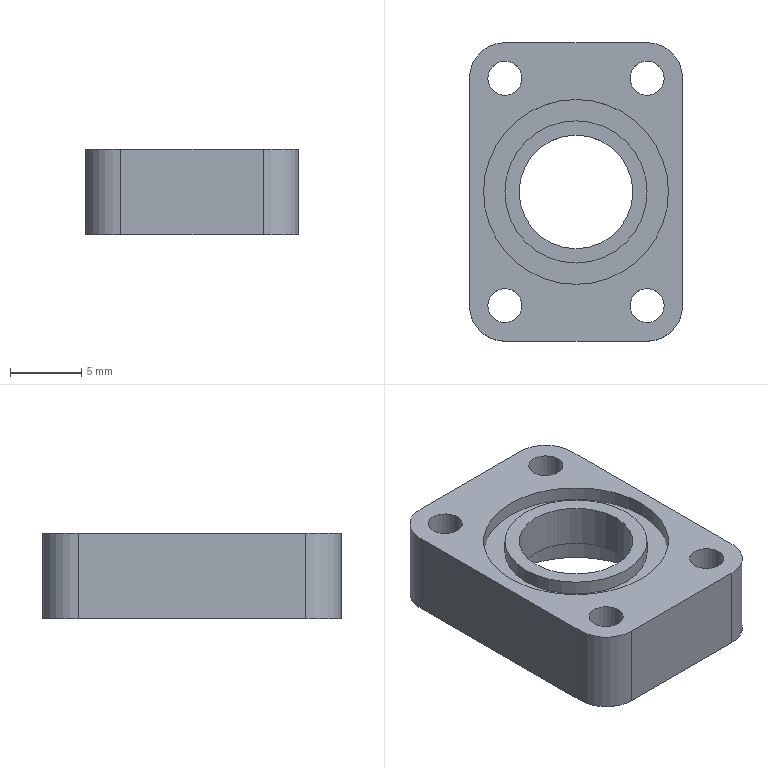Part | SolidWorks | features ICE 5, Extrusion 1, Fillet 1 | 1 solid | 41 faces | box 15 x 21 x 6 mm | volume 975.148 mm3 | cylinder 28 | plane 13 | commonest cylinder face diameters 2.4 x8 4.4 x8 5 x4 13 x4 8 x2 10 x2
STEP:
#1=CARTESIAN_POINT('',(-2.8,8.,4.));
#2=VERTEX_POINT('',#1);
#3=CARTESIAN_POINT('',(-7.2,8.,4.));
#4=VERTEX_POINT('',#3);
#5=CARTESIAN_POINT('',(-5.,8.,4.));
#6=DIRECTION('',(0.,0.,-1.));
#7=DIRECTION('',(-1.,0.,0.));
#8=AXIS2_PLACEMENT_3D('',#5,#6,#7);
#9=CIRCLE('',#8,2.2);
#10=EDGE_CURVE('',#2,#4,#9,.T.);
#11=ORIENTED_EDGE('',*,*,#10,.F.);
#12=CARTESIAN_POINT('',(-2.8,8.,0.));
#13=VERTEX_POINT('',#12);
#14=CARTESIAN_POINT('',(-2.8,8.,4.));
#15=DIRECTION('',(0.,0.,-1.));
#16=VECTOR('',#15,1000.);
#17=LINE('',#14,#16);
#18=EDGE_CURVE('',#2,#13,#17,.T.);
#19=ORIENTED_EDGE('',*,*,#18,.T.);
#20=CARTESIAN_POINT('',(-7.2,8.,0.));
#21=VERTEX_POINT('',#20);
#22=CARTESIAN_POINT('',(-5.,8.,0.));
#23=DIRECTION('',(0.,0.,-1.));
#24=DIRECTION('',(-1.,0.,0.));
#25=AXIS2_PLACEMENT_3D('',#22,#23,#24);
#26=CIRCLE('',#25,2.2);
#27=EDGE_CURVE('',#13,#21,#26,.T.);
#28=ORIENTED_EDGE('',*,*,#27,.T.);
#29=CARTESIAN_POINT('',(-7.2,8.,4.));
#30=DIRECTION('',(0.,0.,-1.));
#31=VECTOR('',#30,1000.);
#32=LINE('',#29,#31);
#33=EDGE_CURVE('',#4,#21,#32,.T.);
#34=ORIENTED_EDGE('',*,*,#33,.F.);
#35=EDGE_LOOP('',(#11,#19,#28,#34));
#36=FACE_OUTER_BOUND('',#35,.T.);
#37=CARTESIAN_POINT('',(-5.,8.,4.));
#38=DIRECTION('',(0.,0.,-1.));
#39=DIRECTION('',(-1.,0.,0.));
#40=AXIS2_PLACEMENT_3D('',#37,#38,#39);
#41=CYLINDRICAL_SURFACE('',#40,2.2);
#42=ADVANCED_FACE('',(#36),#41,.F.);
#43=CARTESIAN_POINT('',(7.2,8.,4.));
#44=VERTEX_POINT('',#43);
#45=CARTESIAN_POINT('',(2.8,8.,4.));
#46=VERTEX_POINT('',#45);
#47=CARTESIAN_POINT('',(5.,8.,4.));
#48=DIRECTION('',(0.,0.,-1.));
#49=DIRECTION('',(-1.,0.,0.));
#50=AXIS2_PLACEMENT_3D('',#47,#48,#49);
#51=CIRCLE('',#50,2.2);
#52=EDGE_CURVE('',#44,#46,#51,.T.);
#53=ORIENTED_EDGE('',*,*,#52,.F.);
#54=CARTESIAN_POINT('',(7.2,8.,0.));
#55=VERTEX_POINT('',#54);
#56=CARTESIAN_POINT('',(7.2,8.,4.));
#57=DIRECTION('',(0.,0.,-1.));
#58=VECTOR('',#57,1000.);
#59=LINE('',#56,#58);
#60=EDGE_CURVE('',#44,#55,#59,.T.);
#61=ORIENTED_EDGE('',*,*,#60,.T.);
#62=CARTESIAN_POINT('',(2.8,8.,0.));
#63=VERTEX_POINT('',#62);
#64=CARTESIAN_POINT('',(5.,8.,0.));
#65=DIRECTION('',(0.,0.,-1.));
#66=DIRECTION('',(-1.,0.,0.));
#67=AXIS2_PLACEMENT_3D('',#64,#65,#66);
#68=CIRCLE('',#67,2.2);
#69=EDGE_CURVE('',#55,#63,#68,.T.);
#70=ORIENTED_EDGE('',*,*,#69,.T.);
#71=CARTESIAN_POINT('',(2.8,8.,4.));
#72=DIRECTION('',(0.,0.,-1.));
#73=VECTOR('',#72,1000.);
#74=LINE('',#71,#73);
#75=EDGE_CURVE('',#46,#63,#74,.T.);
#76=ORIENTED_EDGE('',*,*,#75,.F.);
#77=EDGE_LOOP('',(#53,#61,#70,#76));
#78=FACE_OUTER_BOUND('',#77,.T.);
#79=CARTESIAN_POINT('',(5.,8.,4.));
#80=DIRECTION('',(0.,0.,-1.));
#81=DIRECTION('',(-1.,0.,0.));
#82=AXIS2_PLACEMENT_3D('',#79,#80,#81);
#83=CYLINDRICAL_SURFACE('',#82,2.2);
#84=ADVANCED_FACE('',(#78),#83,.F.);
#85=CARTESIAN_POINT('',(7.2,-8.,4.));
#86=VERTEX_POINT('',#85);
#87=CARTESIAN_POINT('',(2.8,-8.,4.));
#88=VERTEX_POINT('',#87);
#89=CARTESIAN_POINT('',(5.,-8.,4.));
#90=DIRECTION('',(0.,0.,-1.));
#91=DIRECTION('',(-1.,0.,0.));
#92=AXIS2_PLACEMENT_3D('',#89,#90,#91);
#93=CIRCLE('',#92,2.2);
#94=EDGE_CURVE('',#86,#88,#93,.T.);
#95=ORIENTED_EDGE('',*,*,#94,.F.);
#96=CARTESIAN_POINT('',(7.2,-8.,0.));
#97=VERTEX_POINT('',#96);
#98=CARTESIAN_POINT('',(7.2,-8.,4.));
#99=DIRECTION('',(0.,0.,-1.));
#100=VECTOR('',#99,1000.);
#101=LINE('',#98,#100);
#102=EDGE_CURVE('',#86,#97,#101,.T.);
#103=ORIENTED_EDGE('',*,*,#102,.T.);
#104=CARTESIAN_POINT('',(2.8,-8.,0.));
#105=VERTEX_POINT('',#104);
#106=CARTESIAN_POINT('',(5.,-8.,0.));
#107=DIRECTION('',(0.,0.,-1.));
#108=DIRECTION('',(-1.,0.,0.));
#109=AXIS2_PLACEMENT_3D('',#106,#107,#108);
#110=CIRCLE('',#109,2.2);
#111=EDGE_CURVE('',#97,#105,#110,.T.);
#112=ORIENTED_EDGE('',*,*,#111,.T.);
#113=CARTESIAN_POINT('',(2.8,-8.,4.));
#114=DIRECTION('',(0.,0.,-1.));
#115=VECTOR('',#114,1000.);
#116=LINE('',#113,#115);
#117=EDGE_CURVE('',#88,#105,#116,.T.);
#118=ORIENTED_EDGE('',*,*,#117,.F.);
#119=EDGE_LOOP('',(#95,#103,#112,#118));
#120=FACE_OUTER_BOUND('',#119,.T.);
#121=CARTESIAN_POINT('',(5.,-8.,4.));
#122=DIRECTION('',(0.,0.,-1.));
#123=DIRECTION('',(-1.,0.,0.));
#124=AXIS2_PLACEMENT_3D('',#121,#122,#123);
#125=CYLINDRICAL_SURFACE('',#124,2.2);
#126=ADVANCED_FACE('',(#120),#125,.F.);
#127=CARTESIAN_POINT('',(-2.8,-8.,4.));
#128=VERTEX_POINT('',#127);
#129=CARTESIAN_POINT('',(-7.2,-8.,4.));
#130=VERTEX_POINT('',#129);
#131=CARTESIAN_POINT('',(-5.,-8.,4.));
#132=DIRECTION('',(0.,0.,-1.));
#133=DIRECTION('',(-1.,0.,0.));
#134=AXIS2_PLACEMENT_3D('',#131,#132,#133);
#135=CIRCLE('',#134,2.2);
#136=EDGE_CURVE('',#128,#130,#135,.T.);
#137=ORIENTED_EDGE('',*,*,#136,.F.);
#138=CARTESIAN_POINT('',(-2.8,-8.,0.));
#139=VERTEX_POINT('',#138);
#140=CARTESIAN_POINT('',(-2.8,-8.,4.));
#141=DIRECTION('',(0.,0.,-1.));
#142=VECTOR('',#141,1000.);
#143=LINE('',#140,#142);
#144=EDGE_CURVE('',#128,#139,#143,.T.);
#145=ORIENTED_EDGE('',*,*,#144,.T.);
#146=CARTESIAN_POINT('',(-7.2,-8.,0.));
#147=VERTEX_POINT('',#146);
#148=CARTESIAN_POINT('',(-5.,-8.,0.));
#149=DIRECTION('',(0.,0.,-1.));
#150=DIRECTION('',(-1.,0.,0.));
#151=AXIS2_PLACEMENT_3D('',#148,#149,#150);
#152=CIRCLE('',#151,2.2);
#153=EDGE_CURVE('',#139,#147,#152,.T.);
#154=ORIENTED_EDGE('',*,*,#153,.T.);
#155=CARTESIAN_POINT('',(-7.2,-8.,4.));
#156=DIRECTION('',(0.,0.,-1.));
#157=VECTOR('',#156,1000.);
#158=LINE('',#155,#157);
#159=EDGE_CURVE('',#130,#147,#158,.T.);
#160=ORIENTED_EDGE('',*,*,#159,.F.);
#161=EDGE_LOOP('',(#137,#145,#154,#160));
#162=FACE_OUTER_BOUND('',#161,.T.);
#163=CARTESIAN_POINT('',(-5.,-8.,4.));
#164=DIRECTION('',(0.,0.,-1.));
#165=DIRECTION('',(-1.,0.,0.));
#166=AXIS2_PLACEMENT_3D('',#163,#164,#165);
#167=CYLINDRICAL_SURFACE('',#166,2.2);
#168=ADVANCED_FACE('',(#162),#167,.F.);
#169=CARTESIAN_POINT('',(5.,0.,5.));
#170=VERTEX_POINT('',#169);
#171=CARTESIAN_POINT('',(-5.,0.,5.));
#172=VERTEX_POINT('',#171);
#173=CARTESIAN_POINT('',(0.,0.,5.));
#174=DIRECTION('',(0.,0.,1.));
#175=DIRECTION('',(1.,0.,0.));
#176=AXIS2_PLACEMENT_3D('',#173,#174,#175);
#177=CIRCLE('',#176,5.);
#178=EDGE_CURVE('',#170,#172,#177,.T.);
#179=ORIENTED_EDGE('',*,*,#178,.T.);
#180=CARTESIAN_POINT('',(-5.,0.,6.));
#181=VERTEX_POINT('',#180);
#182=CARTESIAN_POINT('',(-5.,0.,5.));
#183=DIRECTION('',(0.,0.,1.));
#184=VECTOR('',#183,1000.);
#185=LINE('',#182,#184);
#186=EDGE_CURVE('',#172,#181,#185,.T.);
#187=ORIENTED_EDGE('',*,*,#186,.T.);
#188=CARTESIAN_POINT('',(5.,0.,6.));
#189=VERTEX_POINT('',#188);
#190=CARTESIAN_POINT('',(0.,0.,6.));
#191=DIRECTION('',(0.,0.,1.));
#192=DIRECTION('',(1.,0.,0.));
#193=AXIS2_PLACEMENT_3D('',#190,#191,#192);
#194=CIRCLE('',#193,5.);
#195=EDGE_CURVE('',#189,#181,#194,.T.);
#196=ORIENTED_EDGE('',*,*,#195,.F.);
#197=CARTESIAN_POINT('',(5.,0.,5.));
#198=DIRECTION('',(0.,0.,1.));
#199=VECTOR('',#198,1000.);
#200=LINE('',#197,#199);
#201=EDGE_CURVE('',#170,#189,#200,.T.);
#202=ORIENTED_EDGE('',*,*,#201,.F.);
#203=EDGE_LOOP('',(#179,#187,#196,#202));
#204=FACE_OUTER_BOUND('',#203,.T.);
#205=CARTESIAN_POINT('',(0.,0.,5.));
#206=DIRECTION('',(0.,0.,1.));
#207=DIRECTION('',(1.,0.,0.));
#208=AXIS2_PLACEMENT_3D('',#205,#206,#207);
#209=CYLINDRICAL_SURFACE('',#208,5.);
#210=ADVANCED_FACE('',(#204),#209,.T.);
#211=CARTESIAN_POINT('',(-6.5,0.,5.));
#212=VERTEX_POINT('',#211);
#213=CARTESIAN_POINT('',(6.5,0.,5.));
#214=VERTEX_POINT('',#213);
#215=CARTESIAN_POINT('',(0.,0.,5.));
#216=DIRECTION('',(0.,0.,1.));
#217=DIRECTION('',(1.,0.,0.));
#218=AXIS2_PLACEMENT_3D('',#215,#216,#217);
#219=CIRCLE('',#218,6.5);
#220=EDGE_CURVE('',#212,#214,#219,.T.);
#221=ORIENTED_EDGE('',*,*,#220,.F.);
#222=CARTESIAN_POINT('',(-6.5,0.,6.));
#223=VERTEX_POINT('',#222);
#224=CARTESIAN_POINT('',(-6.5,0.,5.));
#225=DIRECTION('',(0.,0.,1.));
#226=VECTOR('',#225,1000.);
#227=LINE('',#224,#226);
#228=EDGE_CURVE('',#212,#223,#227,.T.);
#229=ORIENTED_EDGE('',*,*,#228,.T.);
#230=CARTESIAN_POINT('',(6.5,0.,6.));
#231=VERTEX_POINT('',#230);
#232=CARTESIAN_POINT('',(0.,0.,6.));
#233=DIRECTION('',(0.,0.,1.));
#234=DIRECTION('',(1.,0.,0.));
#235=AXIS2_PLACEMENT_3D('',#232,#233,#234);
#236=CIRCLE('',#235,6.5);
#237=EDGE_CURVE('',#223,#231,#236,.T.);
#238=ORIENTED_EDGE('',*,*,#237,.T.);
#239=CARTESIAN_POINT('',(6.5,0.,5.));
#240=DIRECTION('',(0.,0.,1.));
#241=VECTOR('',#240,1000.);
#242=LINE('',#239,#241);
#243=EDGE_CURVE('',#214,#231,#242,.T.);
#244=ORIENTED_EDGE('',*,*,#243,.F.);
#245=EDGE_LOOP('',(#221,#229,#238,#244));
#246=FACE_OUTER_BOUND('',#245,.T.);
#247=CARTESIAN_POINT('',(0.,0.,5.));
#248=DIRECTION('',(0.,0.,1.));
#249=DIRECTION('',(1.,0.,0.));
#250=AXIS2_PLACEMENT_3D('',#247,#248,#249);
#251=CYLINDRICAL_SURFACE('',#250,6.5);
#252=ADVANCED_FACE('',(#246),#251,.F.);
#253=CARTESIAN_POINT('',(6.5,0.,3.));
#254=VERTEX_POINT('',#253);
#255=CARTESIAN_POINT('',(-6.5,0.,3.));
#256=VERTEX_POINT('',#255);
#257=CARTESIAN_POINT('',(0.,0.,3.));
#258=DIRECTION('',(0.,0.,-1.));
#259=DIRECTION('',(-1.,0.,0.));
#260=AXIS2_PLACEMENT_3D('',#257,#258,#259);
#261=CIRCLE('',#260,6.5);
#262=EDGE_CURVE('',#254,#256,#261,.T.);
#263=ORIENTED_EDGE('',*,*,#262,.F.);
#264=CARTESIAN_POINT('',(6.5,0.,0.));
#265=VERTEX_POINT('',#264);
#266=CARTESIAN_POINT('',(6.5,0.,3.));
#267=DIRECTION('',(0.,0.,-1.));
#268=VECTOR('',#267,1000.);
#269=LINE('',#266,#268);
#270=EDGE_CURVE('',#254,#265,#269,.T.);
#271=ORIENTED_EDGE('',*,*,#270,.T.);
#272=CARTESIAN_POINT('',(-6.5,0.,0.));
#273=VERTEX_POINT('',#272);
#274=CARTESIAN_POINT('',(0.,0.,0.));
#275=DIRECTION('',(0.,0.,-1.));
#276=DIRECTION('',(-1.,0.,0.));
#277=AXIS2_PLACEMENT_3D('',#274,#275,#276);
#278=CIRCLE('',#277,6.5);
#279=EDGE_CURVE('',#265,#273,#278,.T.);
#280=ORIENTED_EDGE('',*,*,#279,.T.);
#281=CARTESIAN_POINT('',(-6.5,0.,3.));
#282=DIRECTION('',(0.,0.,-1.));
#283=VECTOR('',#282,1000.);
#284=LINE('',#281,#283);
#285=EDGE_CURVE('',#256,#273,#284,.T.);
#286=ORIENTED_EDGE('',*,*,#285,.F.);
#287=EDGE_LOOP('',(#263,#271,#280,#286));
#288=FACE_OUTER_BOUND('',#287,.T.);
#289=CARTESIAN_POINT('',(0.,0.,3.));
#290=DIRECTION('',(0.,0.,-1.));
#291=DIRECTION('',(-1.,0.,0.));
#292=AXIS2_PLACEMENT_3D('',#289,#290,#291);
#293=CYLINDRICAL_SURFACE('',#292,6.5);
#294=ADVANCED_FACE('',(#288),#293,.F.);
#295=CARTESIAN_POINT('',(-4.,0.,6.));
#296=VERTEX_POINT('',#295);
#297=CARTESIAN_POINT('',(4.,0.,6.));
#298=VERTEX_POINT('',#297);
#299=CARTESIAN_POINT('',(0.,0.,6.));
#300=DIRECTION('',(0.,0.,1.));
#301=DIRECTION('',(1.,0.,0.));
#302=AXIS2_PLACEMENT_3D('',#299,#300,#301);
#303=CIRCLE('',#302,4.);
#304=EDGE_CURVE('',#296,#298,#303,.T.);
#305=ORIENTED_EDGE('',*,*,#304,.T.);
#306=CARTESIAN_POINT('',(4.,0.,3.));
#307=VERTEX_POINT('',#306);
#308=CARTESIAN_POINT('',(4.,0.,6.));
#309=DIRECTION('',(0.,0.,-1.));
#310=VECTOR('',#309,1000.);
#311=LINE('',#308,#310);
#312=EDGE_CURVE('',#298,#307,#311,.T.);
#313=ORIENTED_EDGE('',*,*,#312,.T.);
#314=CARTESIAN_POINT('',(-4.,0.,3.));
#315=VERTEX_POINT('',#314);
#316=CARTESIAN_POINT('',(0.,0.,3.));
#317=DIRECTION('',(0.,0.,-1.));
#318=DIRECTION('',(-1.,0.,0.));
#319=AXIS2_PLACEMENT_3D('',#316,#317,#318);
#320=CIRCLE('',#319,4.);
#321=EDGE_CURVE('',#307,#315,#320,.T.);
#322=ORIENTED_EDGE('',*,*,#321,.T.);
#323=CARTESIAN_POINT('',(-4.,0.,6.));
#324=DIRECTION('',(0.,0.,-1.));
#325=VECTOR('',#324,1000.);
#326=LINE('',#323,#325);
#327=EDGE_CURVE('',#296,#315,#326,.T.);
#328=ORIENTED_EDGE('',*,*,#327,.F.);
#329=EDGE_LOOP('',(#305,#313,#322,#328));
#330=FACE_OUTER_BOUND('',#329,.T.);
#331=CARTESIAN_POINT('',(0.,0.,6.));
#332=DIRECTION('',(0.,0.,-1.));
#333=DIRECTION('',(-1.,0.,0.));
#334=AXIS2_PLACEMENT_3D('',#331,#332,#333);
#335=CYLINDRICAL_SURFACE('',#334,4.);
#336=ADVANCED_FACE('',(#330),#335,.F.);
#337=CARTESIAN_POINT('',(-6.2,-8.,6.));
#338=VERTEX_POINT('',#337);
#339=CARTESIAN_POINT('',(-3.8,-8.,6.));
#340=VERTEX_POINT('',#339);
#341=CARTESIAN_POINT('',(-5.,-8.,6.));
#342=DIRECTION('',(0.,0.,1.));
#343=DIRECTION('',(1.,0.,0.));
#344=AXIS2_PLACEMENT_3D('',#341,#342,#343);
#345=CIRCLE('',#344,1.2);
#346=EDGE_CURVE('',#338,#340,#345,.T.);
#347=ORIENTED_EDGE('',*,*,#346,.T.);
#348=CARTESIAN_POINT('',(-3.8,-8.,4.));
#349=VERTEX_POINT('',#348);
#350=CARTESIAN_POINT('',(-3.8,-8.,17.));
#351=DIRECTION('',(0.,0.,-1.));
#352=VECTOR('',#351,1000.);
#353=LINE('',#350,#352);
#354=EDGE_CURVE('',#340,#349,#353,.T.);
#355=ORIENTED_EDGE('',*,*,#354,.T.);
#356=CARTESIAN_POINT('',(-6.2,-8.,4.));
#357=VERTEX_POINT('',#356);
#358=CARTESIAN_POINT('',(-5.,-8.,4.));
#359=DIRECTION('',(0.,0.,1.));
#360=DIRECTION('',(-1.,0.,0.));
#361=AXIS2_PLACEMENT_3D('',#358,#359,#360);
#362=CIRCLE('',#361,1.2);
#363=EDGE_CURVE('',#357,#349,#362,.T.);
#364=ORIENTED_EDGE('',*,*,#363,.F.);
#365=CARTESIAN_POINT('',(-6.2,-8.,17.));
#366=DIRECTION('',(0.,0.,-1.));
#367=VECTOR('',#366,1000.);
#368=LINE('',#365,#367);
#369=EDGE_CURVE('',#338,#357,#368,.T.);
#370=ORIENTED_EDGE('',*,*,#369,.F.);
#371=EDGE_LOOP('',(#347,#355,#364,#370));
#372=FACE_OUTER_BOUND('',#371,.T.);
#373=CARTESIAN_POINT('',(-5.,-8.,17.));
#374=DIRECTION('',(0.,0.,-1.));
#375=DIRECTION('',(-1.,0.,0.));
#376=AXIS2_PLACEMENT_3D('',#373,#374,#375);
#377=CYLINDRICAL_SURFACE('',#376,1.2);
#378=ADVANCED_FACE('',(#372),#377,.F.);
#379=CARTESIAN_POINT('',(3.8,-8.,6.));
#380=VERTEX_POINT('',#379);
#381=CARTESIAN_POINT('',(6.2,-8.,6.));
#382=VERTEX_POINT('',#381);
#383=CARTESIAN_POINT('',(5.,-8.,6.));
#384=DIRECTION('',(0.,0.,1.));
#385=DIRECTION('',(1.,0.,0.));
#386=AXIS2_PLACEMENT_3D('',#383,#384,#385);
#387=CIRCLE('',#386,1.2);
#388=EDGE_CURVE('',#380,#382,#387,.T.);
#389=ORIENTED_EDGE('',*,*,#388,.T.);
#390=CARTESIAN_POINT('',(6.2,-8.,4.));
#391=VERTEX_POINT('',#390);
#392=CARTESIAN_POINT('',(6.2,-8.,17.));
#393=DIRECTION('',(0.,0.,-1.));
#394=VECTOR('',#393,1000.);
#395=LINE('',#392,#394);
#396=EDGE_CURVE('',#382,#391,#395,.T.);
#397=ORIENTED_EDGE('',*,*,#396,.T.);
#398=CARTESIAN_POINT('',(3.8,-8.,4.));
#399=VERTEX_POINT('',#398);
#400=CARTESIAN_POINT('',(5.,-8.,4.));
#401=DIRECTION('',(0.,0.,1.));
#402=DIRECTION('',(-1.,0.,0.));
#403=AXIS2_PLACEMENT_3D('',#400,#401,#402);
#404=CIRCLE('',#403,1.2);
#405=EDGE_CURVE('',#399,#391,#404,.T.);
#406=ORIENTED_EDGE('',*,*,#405,.F.);
#407=CARTESIAN_POINT('',(3.8,-8.,17.));
#408=DIRECTION('',(0.,0.,-1.));
#409=VECTOR('',#408,1000.);
#410=LINE('',#407,#409);
#411=EDGE_CURVE('',#380,#399,#410,.T.);
#412=ORIENTED_EDGE('',*,*,#411,.F.);
#413=EDGE_LOOP('',(#389,#397,#406,#412));
#414=FACE_OUTER_BOUND('',#413,.T.);
#415=CARTESIAN_POINT('',(5.,-8.,17.));
#416=DIRECTION('',(0.,0.,-1.));
#417=DIRECTION('',(-1.,0.,0.));
#418=AXIS2_PLACEMENT_3D('',#415,#416,#417);
#419=CYLINDRICAL_SURFACE('',#418,1.2);
#420=ADVANCED_FACE('',(#414),#419,.F.);
#421=CARTESIAN_POINT('',(3.8,8.,6.));
#422=VERTEX_POINT('',#421);
#423=CARTESIAN_POINT('',(6.2,8.,6.));
#424=VERTEX_POINT('',#423);
#425=CARTESIAN_POINT('',(5.,8.,6.));
#426=DIRECTION('',(0.,0.,1.));
#427=DIRECTION('',(1.,0.,0.));
#428=AXIS2_PLACEMENT_3D('',#425,#426,#427);
#429=CIRCLE('',#428,1.2);
#430=EDGE_CURVE('',#422,#424,#429,.T.);
#431=ORIENTED_EDGE('',*,*,#430,.T.);
#432=CARTESIAN_POINT('',(6.2,8.,4.));
#433=VERTEX_POINT('',#432);
#434=CARTESIAN_POINT('',(6.2,8.,17.));
#435=DIRECTION('',(0.,0.,-1.));
#436=VECTOR('',#435,1000.);
#437=LINE('',#434,#436);
#438=EDGE_CURVE('',#424,#433,#437,.T.);
#439=ORIENTED_EDGE('',*,*,#438,.T.);
#440=CARTESIAN_POINT('',(3.8,8.,4.));
#441=VERTEX_POINT('',#440);
#442=CARTESIAN_POINT('',(5.,8.,4.));
#443=DIRECTION('',(0.,0.,1.));
#444=DIRECTION('',(-1.,0.,0.));
#445=AXIS2_PLACEMENT_3D('',#442,#443,#444);
#446=CIRCLE('',#445,1.2);
#447=EDGE_CURVE('',#441,#433,#446,.T.);
#448=ORIENTED_EDGE('',*,*,#447,.F.);
#449=CARTESIAN_POINT('',(3.8,8.,17.));
#450=DIRECTION('',(0.,0.,-1.));
#451=VECTOR('',#450,1000.);
#452=LINE('',#449,#451);
#453=EDGE_CURVE('',#422,#441,#452,.T.);
#454=ORIENTED_EDGE('',*,*,#453,.F.);
#455=EDGE_LOOP('',(#431,#439,#448,#454));
#456=FACE_OUTER_BOUND('',#455,.T.);
#457=CARTESIAN_POINT('',(5.,8.,17.));
#458=DIRECTION('',(0.,0.,-1.));
#459=DIRECTION('',(-1.,0.,0.));
#460=AXIS2_PLACEMENT_3D('',#457,#458,#459);
#461=CYLINDRICAL_SURFACE('',#460,1.2);
#462=ADVANCED_FACE('',(#456),#461,.F.);
#463=CARTESIAN_POINT('',(-6.2,8.,6.));
#464=VERTEX_POINT('',#463);
#465=CARTESIAN_POINT('',(-3.8,8.,6.));
#466=VERTEX_POINT('',#465);
#467=CARTESIAN_POINT('',(-5.,8.,6.));
#468=DIRECTION('',(0.,0.,1.));
#469=DIRECTION('',(1.,0.,0.));
#470=AXIS2_PLACEMENT_3D('',#467,#468,#469);
#471=CIRCLE('',#470,1.2);
#472=EDGE_CURVE('',#464,#466,#471,.T.);
#473=ORIENTED_EDGE('',*,*,#472,.T.);
#474=CARTESIAN_POINT('',(-3.8,8.,4.));
#475=VERTEX_POINT('',#474);
#476=CARTESIAN_POINT('',(-3.8,8.,17.));
#477=DIRECTION('',(0.,0.,-1.));
#478=VECTOR('',#477,1000.);
#479=LINE('',#476,#478);
#480=EDGE_CURVE('',#466,#475,#479,.T.);
#481=ORIENTED_EDGE('',*,*,#480,.T.);
#482=CARTESIAN_POINT('',(-6.2,8.,4.));
#483=VERTEX_POINT('',#482);
#484=CARTESIAN_POINT('',(-5.,8.,4.));
#485=DIRECTION('',(0.,0.,1.));
#486=DIRECTION('',(-1.,0.,0.));
#487=AXIS2_PLACEMENT_3D('',#484,#485,#486);
#488=CIRCLE('',#487,1.2);
#489=EDGE_CURVE('',#483,#475,#488,.T.);
#490=ORIENTED_EDGE('',*,*,#489,.F.);
#491=CARTESIAN_POINT('',(-6.2,8.,17.));
#492=DIRECTION('',(0.,0.,-1.));
#493=VECTOR('',#492,1000.);
#494=LINE('',#491,#493);
#495=EDGE_CURVE('',#464,#483,#494,.T.);
#496=ORIENTED_EDGE('',*,*,#495,.F.);
#497=EDGE_LOOP('',(#473,#481,#490,#496));
#498=FACE_OUTER_BOUND('',#497,.T.);
#499=CARTESIAN_POINT('',(-5.,8.,17.));
#500=DIRECTION('',(0.,0.,-1.));
#501=DIRECTION('',(-1.,0.,0.));
#502=AXIS2_PLACEMENT_3D('',#499,#500,#501);
#503=CYLINDRICAL_SURFACE('',#502,1.2);
#504=ADVANCED_FACE('',(#498),#503,.F.);
#505=ORIENTED_EDGE('',*,*,#480,.F.);
#506=CARTESIAN_POINT('',(-5.,8.,6.));
#507=DIRECTION('',(0.,0.,1.));
#508=DIRECTION('',(1.,0.,0.));
#509=AXIS2_PLACEMENT_3D('',#506,#507,#508);
#510=CIRCLE('',#509,1.2);
#511=EDGE_CURVE('',#466,#464,#510,.T.);
#512=ORIENTED_EDGE('',*,*,#511,.T.);
#513=ORIENTED_EDGE('',*,*,#495,.T.);
#514=CARTESIAN_POINT('',(-5.,8.,4.));
#515=DIRECTION('',(0.,0.,1.));
#516=DIRECTION('',(-1.,0.,0.));
#517=AXIS2_PLACEMENT_3D('',#514,#515,#516);
#518=CIRCLE('',#517,1.2);
#519=EDGE_CURVE('',#475,#483,#518,.T.);
#520=ORIENTED_EDGE('',*,*,#519,.F.);
#521=EDGE_LOOP('',(#505,#512,#513,#520));
#522=FACE_OUTER_BOUND('',#521,.T.);
#523=CARTESIAN_POINT('',(-5.,8.,17.));
#524=DIRECTION('',(0.,0.,-1.));
#525=DIRECTION('',(-1.,0.,0.));
#526=AXIS2_PLACEMENT_3D('',#523,#524,#525);
#527=CYLINDRICAL_SURFACE('',#526,1.2);
#528=ADVANCED_FACE('',(#522),#527,.F.);
#529=ORIENTED_EDGE('',*,*,#438,.F.);
#530=CARTESIAN_POINT('',(5.,8.,6.));
#531=DIRECTION('',(0.,0.,1.));
#532=DIRECTION('',(1.,0.,0.));
#533=AXIS2_PLACEMENT_3D('',#530,#531,#532);
#534=CIRCLE('',#533,1.2);
#535=EDGE_CURVE('',#424,#422,#534,.T.);
#536=ORIENTED_EDGE('',*,*,#535,.T.);
#537=ORIENTED_EDGE('',*,*,#453,.T.);
#538=CARTESIAN_POINT('',(5.,8.,4.));
#539=DIRECTION('',(0.,0.,1.));
#540=DIRECTION('',(-1.,0.,0.));
#541=AXIS2_PLACEMENT_3D('',#538,#539,#540);
#542=CIRCLE('',#541,1.2);
#543=EDGE_CURVE('',#433,#441,#542,.T.);
#544=ORIENTED_EDGE('',*,*,#543,.F.);
#545=EDGE_LOOP('',(#529,#536,#537,#544));
#546=FACE_OUTER_BOUND('',#545,.T.);
#547=CARTESIAN_POINT('',(5.,8.,17.));
#548=DIRECTION('',(0.,0.,-1.));
#549=DIRECTION('',(-1.,0.,0.));
#550=AXIS2_PLACEMENT_3D('',#547,#548,#549);
#551=CYLINDRICAL_SURFACE('',#550,1.2);
#552=ADVANCED_FACE('',(#546),#551,.F.);
#553=ORIENTED_EDGE('',*,*,#396,.F.);
#554=CARTESIAN_POINT('',(5.,-8.,6.));
#555=DIRECTION('',(0.,0.,1.));
#556=DIRECTION('',(1.,0.,0.));
#557=AXIS2_PLACEMENT_3D('',#554,#555,#556);
#558=CIRCLE('',#557,1.2);
#559=EDGE_CURVE('',#382,#380,#558,.T.);
#560=ORIENTED_EDGE('',*,*,#559,.T.);
#561=ORIENTED_EDGE('',*,*,#411,.T.);
#562=CARTESIAN_POINT('',(5.,-8.,4.));
#563=DIRECTION('',(0.,0.,1.));
#564=DIRECTION('',(-1.,0.,0.));
#565=AXIS2_PLACEMENT_3D('',#562,#563,#564);
#566=CIRCLE('',#565,1.2);
#567=EDGE_CURVE('',#391,#399,#566,.T.);
#568=ORIENTED_EDGE('',*,*,#567,.F.);
#569=EDGE_LOOP('',(#553,#560,#561,#568));
#570=FACE_OUTER_BOUND('',#569,.T.);
#571=CARTESIAN_POINT('',(5.,-8.,17.));
#572=DIRECTION('',(0.,0.,-1.));
#573=DIRECTION('',(-1.,0.,0.));
#574=AXIS2_PLACEMENT_3D('',#571,#572,#573);
#575=CYLINDRICAL_SURFACE('',#574,1.2);
#576=ADVANCED_FACE('',(#570),#575,.F.);
#577=ORIENTED_EDGE('',*,*,#354,.F.);
#578=CARTESIAN_POINT('',(-5.,-8.,6.));
#579=DIRECTION('',(0.,0.,1.));
#580=DIRECTION('',(1.,0.,0.));
#581=AXIS2_PLACEMENT_3D('',#578,#579,#580);
#582=CIRCLE('',#581,1.2);
#583=EDGE_CURVE('',#340,#338,#582,.T.);
#584=ORIENTED_EDGE('',*,*,#583,.T.);
#585=ORIENTED_EDGE('',*,*,#369,.T.);
#586=CARTESIAN_POINT('',(-5.,-8.,4.));
#587=DIRECTION('',(0.,0.,1.));
#588=DIRECTION('',(-1.,0.,0.));
#589=AXIS2_PLACEMENT_3D('',#586,#587,#588);
#590=CIRCLE('',#589,1.2);
#591=EDGE_CURVE('',#349,#357,#590,.T.);
#592=ORIENTED_EDGE('',*,*,#591,.F.);
#593=EDGE_LOOP('',(#577,#584,#585,#592));
#594=FACE_OUTER_BOUND('',#593,.T.);
#595=CARTESIAN_POINT('',(-5.,-8.,17.));
#596=DIRECTION('',(0.,0.,-1.));
#597=DIRECTION('',(-1.,0.,0.));
#598=AXIS2_PLACEMENT_3D('',#595,#596,#597);
#599=CYLINDRICAL_SURFACE('',#598,1.2);
#600=ADVANCED_FACE('',(#594),#599,.F.);
#601=ORIENTED_EDGE('',*,*,#304,.F.);
#602=CARTESIAN_POINT('',(0.,0.,6.));
#603=DIRECTION('',(0.,0.,1.));
#604=DIRECTION('',(1.,0.,0.));
#605=AXIS2_PLACEMENT_3D('',#602,#603,#604);
#606=CIRCLE('',#605,4.);
#607=EDGE_CURVE('',#298,#296,#606,.T.);
#608=ORIENTED_EDGE('',*,*,#607,.F.);
#609=EDGE_LOOP('',(#601,#608));
#610=FACE_BOUND('',#609,.T.);
#611=ORIENTED_EDGE('',*,*,#195,.T.);
#612=CARTESIAN_POINT('',(0.,0.,6.));
#613=DIRECTION('',(0.,0.,1.));
#614=DIRECTION('',(1.,0.,0.));
#615=AXIS2_PLACEMENT_3D('',#612,#613,#614);
#616=CIRCLE('',#615,5.);
#617=EDGE_CURVE('',#181,#189,#616,.T.);
#618=ORIENTED_EDGE('',*,*,#617,.T.);
#619=EDGE_LOOP('',(#611,#618));
#620=FACE_OUTER_BOUND('',#619,.T.);
#621=CARTESIAN_POINT('',(0.,0.,6.));
#622=DIRECTION('',(0.,0.,1.));
#623=DIRECTION('',(1.,0.,0.));
#624=AXIS2_PLACEMENT_3D('',#621,#622,#623);
#625=PLANE('',#624);
#626=ADVANCED_FACE('',(#610,#620),#625,.T.);
#627=ORIENTED_EDGE('',*,*,#312,.F.);
#628=ORIENTED_EDGE('',*,*,#607,.T.);
#629=ORIENTED_EDGE('',*,*,#327,.T.);
#630=CARTESIAN_POINT('',(0.,0.,3.));
#631=DIRECTION('',(0.,0.,-1.));
#632=DIRECTION('',(-1.,0.,0.));
#633=AXIS2_PLACEMENT_3D('',#630,#631,#632);
#634=CIRCLE('',#633,4.);
#635=EDGE_CURVE('',#315,#307,#634,.T.);
#636=ORIENTED_EDGE('',*,*,#635,.T.);
#637=EDGE_LOOP('',(#627,#628,#629,#636));
#638=FACE_OUTER_BOUND('',#637,.T.);
#639=CARTESIAN_POINT('',(0.,0.,6.));
#640=DIRECTION('',(0.,0.,-1.));
#641=DIRECTION('',(-1.,0.,0.));
#642=AXIS2_PLACEMENT_3D('',#639,#640,#641);
#643=CYLINDRICAL_SURFACE('',#642,4.);
#644=ADVANCED_FACE('',(#638),#643,.F.);
#645=ORIENTED_EDGE('',*,*,#346,.F.);
#646=ORIENTED_EDGE('',*,*,#583,.F.);
#647=EDGE_LOOP('',(#645,#646));
#648=FACE_BOUND('',#647,.T.);
#649=ORIENTED_EDGE('',*,*,#388,.F.);
#650=ORIENTED_EDGE('',*,*,#559,.F.);
#651=EDGE_LOOP('',(#649,#650));
#652=FACE_BOUND('',#651,.T.);
#653=ORIENTED_EDGE('',*,*,#430,.F.);
#654=ORIENTED_EDGE('',*,*,#535,.F.);
#655=EDGE_LOOP('',(#653,#654));
#656=FACE_BOUND('',#655,.T.);
#657=ORIENTED_EDGE('',*,*,#472,.F.);
#658=ORIENTED_EDGE('',*,*,#511,.F.);
#659=EDGE_LOOP('',(#657,#658));
#660=FACE_BOUND('',#659,.T.);
#661=CARTESIAN_POINT('',(0.,0.,6.));
#662=DIRECTION('',(0.,0.,1.));
#663=DIRECTION('',(1.,0.,0.));
#664=AXIS2_PLACEMENT_3D('',#661,#662,#663);
#665=CIRCLE('',#664,6.5);
#666=EDGE_CURVE('',#231,#223,#665,.T.);
#667=ORIENTED_EDGE('',*,*,#666,.F.);
#668=ORIENTED_EDGE('',*,*,#237,.F.);
#669=EDGE_LOOP('',(#667,#668));
#670=FACE_BOUND('',#669,.T.);
#671=CARTESIAN_POINT('',(-5.,10.5,6.));
#672=VERTEX_POINT('',#671);
#673=CARTESIAN_POINT('',(5.,10.5,6.));
#674=VERTEX_POINT('',#673);
#675=CARTESIAN_POINT('',(7.5,10.5,6.));
#676=DIRECTION('',(1.,0.,0.));
#677=VECTOR('',#676,1000.);
#678=LINE('',#675,#677);
#679=EDGE_CURVE('',#672,#674,#678,.T.);
#680=ORIENTED_EDGE('',*,*,#679,.F.);
#681=CARTESIAN_POINT('',(-7.5,8.,6.));
#682=VERTEX_POINT('',#681);
#683=CARTESIAN_POINT('',(-5.,8.,6.));
#684=DIRECTION('',(0.,0.,1.));
#685=DIRECTION('',(1.,0.,0.));
#686=AXIS2_PLACEMENT_3D('',#683,#684,#685);
#687=CIRCLE('',#686,2.5);
#688=EDGE_CURVE('',#672,#682,#687,.T.);
#689=ORIENTED_EDGE('',*,*,#688,.T.);
#690=CARTESIAN_POINT('',(-7.5,-8.,6.));
#691=VERTEX_POINT('',#690);
#692=CARTESIAN_POINT('',(-7.5,7.5,6.));
#693=DIRECTION('',(0.,-1.,0.));
#694=VECTOR('',#693,1000.);
#695=LINE('',#692,#694);
#696=EDGE_CURVE('',#682,#691,#695,.T.);
#697=ORIENTED_EDGE('',*,*,#696,.T.);
#698=CARTESIAN_POINT('',(-5.,-10.5,6.));
#699=VERTEX_POINT('',#698);
#700=CARTESIAN_POINT('',(-5.,-8.,6.));
#701=DIRECTION('',(0.,0.,1.));
#702=DIRECTION('',(1.,0.,0.));
#703=AXIS2_PLACEMENT_3D('',#700,#701,#702);
#704=CIRCLE('',#703,2.5);
#705=EDGE_CURVE('',#691,#699,#704,.T.);
#706=ORIENTED_EDGE('',*,*,#705,.T.);
#707=CARTESIAN_POINT('',(5.,-10.5,6.));
#708=VERTEX_POINT('',#707);
#709=CARTESIAN_POINT('',(-7.5,-10.5,6.));
#710=DIRECTION('',(-1.,0.,0.));
#711=VECTOR('',#710,1000.);
#712=LINE('',#709,#711);
#713=EDGE_CURVE('',#708,#699,#712,.T.);
#714=ORIENTED_EDGE('',*,*,#713,.F.);
#715=CARTESIAN_POINT('',(7.5,-8.,6.));
#716=VERTEX_POINT('',#715);
#717=CARTESIAN_POINT('',(5.,-8.,6.));
#718=DIRECTION('',(0.,0.,1.));
#719=DIRECTION('',(1.,0.,0.));
#720=AXIS2_PLACEMENT_3D('',#717,#718,#719);
#721=CIRCLE('',#720,2.5);
#722=EDGE_CURVE('',#708,#716,#721,.T.);
#723=ORIENTED_EDGE('',*,*,#722,.T.);
#724=CARTESIAN_POINT('',(7.5,8.,6.));
#725=VERTEX_POINT('',#724);
#726=CARTESIAN_POINT('',(7.5,-7.5,6.));
#727=DIRECTION('',(0.,1.,0.));
#728=VECTOR('',#727,1000.);
#729=LINE('',#726,#728);
#730=EDGE_CURVE('',#716,#725,#729,.T.);
#731=ORIENTED_EDGE('',*,*,#730,.T.);
#732=CARTESIAN_POINT('',(5.,8.,6.));
#733=DIRECTION('',(0.,0.,1.));
#734=DIRECTION('',(1.,0.,0.));
#735=AXIS2_PLACEMENT_3D('',#732,#733,#734);
#736=CIRCLE('',#735,2.5);
#737=EDGE_CURVE('',#725,#674,#736,.T.);
#738=ORIENTED_EDGE('',*,*,#737,.T.);
#739=EDGE_LOOP('',(#680,#689,#697,#706,#714,#723,#731,#738));
#740=FACE_OUTER_BOUND('',#739,.T.);
#741=CARTESIAN_POINT('',(0.,0.,6.));
#742=DIRECTION('',(0.,0.,1.));
#743=DIRECTION('',(1.,0.,0.));
#744=AXIS2_PLACEMENT_3D('',#741,#742,#743);
#745=PLANE('',#744);
#746=ADVANCED_FACE('',(#648,#652,#656,#660,#670,#740),#745,.T.);
#747=CARTESIAN_POINT('',(-5.,-8.,0.));
#748=DIRECTION('',(0.,0.,-1.));
#749=DIRECTION('',(-1.,0.,0.));
#750=AXIS2_PLACEMENT_3D('',#747,#748,#749);
#751=CIRCLE('',#750,2.2);
#752=EDGE_CURVE('',#147,#139,#751,.T.);
#753=ORIENTED_EDGE('',*,*,#752,.F.);
#754=ORIENTED_EDGE('',*,*,#153,.F.);
#755=EDGE_LOOP('',(#753,#754));
#756=FACE_BOUND('',#755,.T.);
#757=CARTESIAN_POINT('',(-5.,8.,0.));
#758=DIRECTION('',(0.,0.,-1.));
#759=DIRECTION('',(-1.,0.,0.));
#760=AXIS2_PLACEMENT_3D('',#757,#758,#759);
#761=CIRCLE('',#760,2.2);
#762=EDGE_CURVE('',#21,#13,#761,.T.);
#763=ORIENTED_EDGE('',*,*,#762,.F.);
#764=ORIENTED_EDGE('',*,*,#27,.F.);
#765=EDGE_LOOP('',(#763,#764));
#766=FACE_BOUND('',#765,.T.);
#767=CARTESIAN_POINT('',(5.,8.,0.));
#768=DIRECTION('',(0.,0.,-1.));
#769=DIRECTION('',(-1.,0.,0.));
#770=AXIS2_PLACEMENT_3D('',#767,#768,#769);
#771=CIRCLE('',#770,2.2);
#772=EDGE_CURVE('',#63,#55,#771,.T.);
#773=ORIENTED_EDGE('',*,*,#772,.F.);
#774=ORIENTED_EDGE('',*,*,#69,.F.);
#775=EDGE_LOOP('',(#773,#774));
#776=FACE_BOUND('',#775,.T.);
#777=CARTESIAN_POINT('',(5.,-8.,0.));
#778=DIRECTION('',(0.,0.,-1.));
#779=DIRECTION('',(-1.,0.,0.));
#780=AXIS2_PLACEMENT_3D('',#777,#778,#779);
#781=CIRCLE('',#780,2.2);
#782=EDGE_CURVE('',#105,#97,#781,.T.);
#783=ORIENTED_EDGE('',*,*,#782,.F.);
#784=ORIENTED_EDGE('',*,*,#111,.F.);
#785=EDGE_LOOP('',(#783,#784));
#786=FACE_BOUND('',#785,.T.);
#787=CARTESIAN_POINT('',(0.,0.,0.));
#788=DIRECTION('',(0.,0.,-1.));
#789=DIRECTION('',(-1.,0.,0.));
#790=AXIS2_PLACEMENT_3D('',#787,#788,#789);
#791=CIRCLE('',#790,6.5);
#792=EDGE_CURVE('',#273,#265,#791,.T.);
#793=ORIENTED_EDGE('',*,*,#792,.F.);
#794=ORIENTED_EDGE('',*,*,#279,.F.);
#795=EDGE_LOOP('',(#793,#794));
#796=FACE_BOUND('',#795,.T.);
#797=CARTESIAN_POINT('',(-7.5,8.,0.));
#798=VERTEX_POINT('',#797);
#799=CARTESIAN_POINT('',(-7.5,-8.,0.));
#800=VERTEX_POINT('',#799);
#801=CARTESIAN_POINT('',(-7.5,7.5,0.));
#802=DIRECTION('',(0.,-1.,0.));
#803=VECTOR('',#802,1000.);
#804=LINE('',#801,#803);
#805=EDGE_CURVE('',#798,#800,#804,.T.);
#806=ORIENTED_EDGE('',*,*,#805,.F.);
#807=CARTESIAN_POINT('',(-5.,10.5,0.));
#808=VERTEX_POINT('',#807);
#809=CARTESIAN_POINT('',(-5.,8.,0.));
#810=DIRECTION('',(0.,0.,-1.));
#811=DIRECTION('',(1.,0.,0.));
#812=AXIS2_PLACEMENT_3D('',#809,#810,#811);
#813=CIRCLE('',#812,2.5);
#814=EDGE_CURVE('',#798,#808,#813,.T.);
#815=ORIENTED_EDGE('',*,*,#814,.T.);
#816=CARTESIAN_POINT('',(5.,10.5,0.));
#817=VERTEX_POINT('',#816);
#818=CARTESIAN_POINT('',(7.5,10.5,0.));
#819=DIRECTION('',(1.,0.,0.));
#820=VECTOR('',#819,1000.);
#821=LINE('',#818,#820);
#822=EDGE_CURVE('',#808,#817,#821,.T.);
#823=ORIENTED_EDGE('',*,*,#822,.T.);
#824=CARTESIAN_POINT('',(7.5,8.,0.));
#825=VERTEX_POINT('',#824);
#826=CARTESIAN_POINT('',(5.,8.,0.));
#827=DIRECTION('',(0.,0.,-1.));
#828=DIRECTION('',(1.,0.,0.));
#829=AXIS2_PLACEMENT_3D('',#826,#827,#828);
#830=CIRCLE('',#829,2.5);
#831=EDGE_CURVE('',#817,#825,#830,.T.);
#832=ORIENTED_EDGE('',*,*,#831,.T.);
#833=CARTESIAN_POINT('',(7.5,-8.,0.));
#834=VERTEX_POINT('',#833);
#835=CARTESIAN_POINT('',(7.5,0.,0.));
#836=DIRECTION('',(0.,1.,0.));
#837=VECTOR('',#836,1000.);
#838=LINE('',#835,#837);
#839=EDGE_CURVE('',#834,#825,#838,.T.);
#840=ORIENTED_EDGE('',*,*,#839,.F.);
#841=CARTESIAN_POINT('',(5.,-10.5,0.));
#842=VERTEX_POINT('',#841);
#843=CARTESIAN_POINT('',(5.,-8.,0.));
#844=DIRECTION('',(0.,0.,-1.));
#845=DIRECTION('',(1.,0.,0.));
#846=AXIS2_PLACEMENT_3D('',#843,#844,#845);
#847=CIRCLE('',#846,2.5);
#848=EDGE_CURVE('',#834,#842,#847,.T.);
#849=ORIENTED_EDGE('',*,*,#848,.T.);
#850=CARTESIAN_POINT('',(-5.,-10.5,0.));
#851=VERTEX_POINT('',#850);
#852=CARTESIAN_POINT('',(-7.5,-10.5,0.));
#853=DIRECTION('',(-1.,0.,0.));
#854=VECTOR('',#853,1000.);
#855=LINE('',#852,#854);
#856=EDGE_CURVE('',#842,#851,#855,.T.);
#857=ORIENTED_EDGE('',*,*,#856,.T.);
#858=CARTESIAN_POINT('',(-5.,-8.,0.));
#859=DIRECTION('',(0.,0.,-1.));
#860=DIRECTION('',(1.,0.,0.));
#861=AXIS2_PLACEMENT_3D('',#858,#859,#860);
#862=CIRCLE('',#861,2.5);
#863=EDGE_CURVE('',#851,#800,#862,.T.);
#864=ORIENTED_EDGE('',*,*,#863,.T.);
#865=EDGE_LOOP('',(#806,#815,#823,#832,#840,#849,#857,#864));
#866=FACE_OUTER_BOUND('',#865,.T.);
#867=CARTESIAN_POINT('',(0.,0.,0.));
#868=DIRECTION('',(0.,0.,1.));
#869=DIRECTION('',(1.,0.,0.));
#870=AXIS2_PLACEMENT_3D('',#867,#868,#869);
#871=PLANE('',#870);
#872=ADVANCED_FACE('',(#756,#766,#776,#786,#796,#866),#871,.F.);
#873=ORIENTED_EDGE('',*,*,#696,.F.);
#874=CARTESIAN_POINT('',(-7.5,8.,0.));
#875=DIRECTION('',(0.,0.,-1.));
#876=VECTOR('',#875,1000.);
#877=LINE('',#874,#876);
#878=EDGE_CURVE('',#682,#798,#877,.T.);
#879=ORIENTED_EDGE('',*,*,#878,.T.);
#880=ORIENTED_EDGE('',*,*,#805,.T.);
#881=CARTESIAN_POINT('',(-7.5,-8.,6.));
#882=DIRECTION('',(0.,0.,1.));
#883=VECTOR('',#882,1000.);
#884=LINE('',#881,#883);
#885=EDGE_CURVE('',#800,#691,#884,.T.);
#886=ORIENTED_EDGE('',*,*,#885,.T.);
#887=EDGE_LOOP('',(#873,#879,#880,#886));
#888=FACE_OUTER_BOUND('',#887,.T.);
#889=CARTESIAN_POINT('',(-7.5,7.5,6.));
#890=DIRECTION('',(1.,0.,0.));
#891=DIRECTION('',(0.,1.,0.));
#892=AXIS2_PLACEMENT_3D('',#889,#890,#891);
#893=PLANE('',#892);
#894=ADVANCED_FACE('',(#888),#893,.F.);
#895=ORIENTED_EDGE('',*,*,#730,.F.);
#896=CARTESIAN_POINT('',(7.5,-8.,0.));
#897=DIRECTION('',(0.,0.,-1.));
#898=VECTOR('',#897,1000.);
#899=LINE('',#896,#898);
#900=EDGE_CURVE('',#716,#834,#899,.T.);
#901=ORIENTED_EDGE('',*,*,#900,.T.);
#902=ORIENTED_EDGE('',*,*,#839,.T.);
#903=CARTESIAN_POINT('',(7.5,8.,6.));
#904=DIRECTION('',(0.,0.,1.));
#905=VECTOR('',#904,1000.);
#906=LINE('',#903,#905);
#907=EDGE_CURVE('',#825,#725,#906,.T.);
#908=ORIENTED_EDGE('',*,*,#907,.T.);
#909=EDGE_LOOP('',(#895,#901,#902,#908));
#910=FACE_OUTER_BOUND('',#909,.T.);
#911=CARTESIAN_POINT('',(7.5,0.,6.));
#912=DIRECTION('',(-1.,0.,0.));
#913=DIRECTION('',(0.,0.,1.));
#914=AXIS2_PLACEMENT_3D('',#911,#912,#913);
#915=PLANE('',#914);
#916=ADVANCED_FACE('',(#910),#915,.F.);
#917=ORIENTED_EDGE('',*,*,#270,.F.);
#918=CARTESIAN_POINT('',(0.,0.,3.));
#919=DIRECTION('',(0.,0.,-1.));
#920=DIRECTION('',(-1.,0.,0.));
#921=AXIS2_PLACEMENT_3D('',#918,#919,#920);
#922=CIRCLE('',#921,6.5);
#923=EDGE_CURVE('',#256,#254,#922,.T.);
#924=ORIENTED_EDGE('',*,*,#923,.F.);
#925=ORIENTED_EDGE('',*,*,#285,.T.);
#926=ORIENTED_EDGE('',*,*,#792,.T.);
#927=EDGE_LOOP('',(#917,#924,#925,#926));
#928=FACE_OUTER_BOUND('',#927,.T.);
#929=CARTESIAN_POINT('',(0.,0.,3.));
#930=DIRECTION('',(0.,0.,-1.));
#931=DIRECTION('',(-1.,0.,0.));
#932=AXIS2_PLACEMENT_3D('',#929,#930,#931);
#933=CYLINDRICAL_SURFACE('',#932,6.5);
#934=ADVANCED_FACE('',(#928),#933,.F.);
#935=ORIENTED_EDGE('',*,*,#635,.F.);
#936=ORIENTED_EDGE('',*,*,#321,.F.);
#937=EDGE_LOOP('',(#935,#936));
#938=FACE_BOUND('',#937,.T.);
#939=ORIENTED_EDGE('',*,*,#923,.T.);
#940=ORIENTED_EDGE('',*,*,#262,.T.);
#941=EDGE_LOOP('',(#939,#940));
#942=FACE_OUTER_BOUND('',#941,.T.);
#943=CARTESIAN_POINT('',(0.,0.,3.));
#944=DIRECTION('',(0.,0.,-1.));
#945=DIRECTION('',(-1.,0.,0.));
#946=AXIS2_PLACEMENT_3D('',#943,#944,#945);
#947=PLANE('',#946);
#948=ADVANCED_FACE('',(#938,#942),#947,.T.);
#949=ORIENTED_EDGE('',*,*,#228,.F.);
#950=CARTESIAN_POINT('',(0.,0.,5.));
#951=DIRECTION('',(0.,0.,1.));
#952=DIRECTION('',(1.,0.,0.));
#953=AXIS2_PLACEMENT_3D('',#950,#951,#952);
#954=CIRCLE('',#953,6.5);
#955=EDGE_CURVE('',#214,#212,#954,.T.);
#956=ORIENTED_EDGE('',*,*,#955,.F.);
#957=ORIENTED_EDGE('',*,*,#243,.T.);
#958=ORIENTED_EDGE('',*,*,#666,.T.);
#959=EDGE_LOOP('',(#949,#956,#957,#958));
#960=FACE_OUTER_BOUND('',#959,.T.);
#961=CARTESIAN_POINT('',(0.,0.,5.));
#962=DIRECTION('',(0.,0.,1.));
#963=DIRECTION('',(1.,0.,0.));
#964=AXIS2_PLACEMENT_3D('',#961,#962,#963);
#965=CYLINDRICAL_SURFACE('',#964,6.5);
#966=ADVANCED_FACE('',(#960),#965,.F.);
#967=ORIENTED_EDGE('',*,*,#178,.F.);
#968=CARTESIAN_POINT('',(0.,0.,5.));
#969=DIRECTION('',(0.,0.,1.));
#970=DIRECTION('',(1.,0.,0.));
#971=AXIS2_PLACEMENT_3D('',#968,#969,#970);
#972=CIRCLE('',#971,5.);
#973=EDGE_CURVE('',#172,#170,#972,.T.);
#974=ORIENTED_EDGE('',*,*,#973,.F.);
#975=EDGE_LOOP('',(#967,#974));
#976=FACE_BOUND('',#975,.T.);
#977=ORIENTED_EDGE('',*,*,#955,.T.);
#978=ORIENTED_EDGE('',*,*,#220,.T.);
#979=EDGE_LOOP('',(#977,#978));
#980=FACE_OUTER_BOUND('',#979,.T.);
#981=CARTESIAN_POINT('',(0.,0.,5.));
#982=DIRECTION('',(0.,0.,1.));
#983=DIRECTION('',(1.,0.,0.));
#984=AXIS2_PLACEMENT_3D('',#981,#982,#983);
#985=PLANE('',#984);
#986=ADVANCED_FACE('',(#976,#980),#985,.T.);
#987=ORIENTED_EDGE('',*,*,#186,.F.);
#988=ORIENTED_EDGE('',*,*,#973,.T.);
#989=ORIENTED_EDGE('',*,*,#201,.T.);
#990=ORIENTED_EDGE('',*,*,#617,.F.);
#991=EDGE_LOOP('',(#987,#988,#989,#990));
#992=FACE_OUTER_BOUND('',#991,.T.);
#993=CARTESIAN_POINT('',(0.,0.,5.));
#994=DIRECTION('',(0.,0.,1.));
#995=DIRECTION('',(1.,0.,0.));
#996=AXIS2_PLACEMENT_3D('',#993,#994,#995);
#997=CYLINDRICAL_SURFACE('',#996,5.);
#998=ADVANCED_FACE('',(#992),#997,.T.);
#999=ORIENTED_EDGE('',*,*,#713,.T.);
#1000=CARTESIAN_POINT('',(-5.,-10.5,0.));
#1001=DIRECTION('',(0.,0.,-1.));
#1002=VECTOR('',#1001,1000.);
#1003=LINE('',#1000,#1002);
#1004=EDGE_CURVE('',#699,#851,#1003,.T.);
#1005=ORIENTED_EDGE('',*,*,#1004,.T.);
#1006=ORIENTED_EDGE('',*,*,#856,.F.);
#1007=CARTESIAN_POINT('',(5.,-10.5,6.));
#1008=DIRECTION('',(0.,0.,1.));
#1009=VECTOR('',#1008,1000.);
#1010=LINE('',#1007,#1009);
#1011=EDGE_CURVE('',#842,#708,#1010,.T.);
#1012=ORIENTED_EDGE('',*,*,#1011,.T.);
#1013=EDGE_LOOP('',(#999,#1005,#1006,#1012));
#1014=FACE_OUTER_BOUND('',#1013,.T.);
#1015=CARTESIAN_POINT('',(-7.5,-10.5,6.));
#1016=DIRECTION('',(0.,-1.,0.));
#1017=DIRECTION('',(1.,0.,0.));
#1018=AXIS2_PLACEMENT_3D('',#1015,#1016,#1017);
#1019=PLANE('',#1018);
#1020=ADVANCED_FACE('',(#1014),#1019,.T.);
#1021=ORIENTED_EDGE('',*,*,#822,.F.);
#1022=CARTESIAN_POINT('',(-5.,10.5,6.));
#1023=DIRECTION('',(0.,0.,1.));
#1024=VECTOR('',#1023,1000.);
#1025=LINE('',#1022,#1024);
#1026=EDGE_CURVE('',#808,#672,#1025,.T.);
#1027=ORIENTED_EDGE('',*,*,#1026,.T.);
#1028=ORIENTED_EDGE('',*,*,#679,.T.);
#1029=CARTESIAN_POINT('',(5.,10.5,0.));
#1030=DIRECTION('',(0.,0.,-1.));
#1031=VECTOR('',#1030,1000.);
#1032=LINE('',#1029,#1031);
#1033=EDGE_CURVE('',#674,#817,#1032,.T.);
#1034=ORIENTED_EDGE('',*,*,#1033,.T.);
#1035=EDGE_LOOP('',(#1021,#1027,#1028,#1034));
#1036=FACE_OUTER_BOUND('',#1035,.T.);
#1037=CARTESIAN_POINT('',(7.5,10.5,6.));
#1038=DIRECTION('',(0.,1.,0.));
#1039=DIRECTION('',(0.,0.,1.));
#1040=AXIS2_PLACEMENT_3D('',#1037,#1038,#1039);
#1041=PLANE('',#1040);
#1042=ADVANCED_FACE('',(#1036),#1041,.T.);
#1043=ORIENTED_EDGE('',*,*,#688,.F.);
#1044=ORIENTED_EDGE('',*,*,#1026,.F.);
#1045=ORIENTED_EDGE('',*,*,#814,.F.);
#1046=ORIENTED_EDGE('',*,*,#878,.F.);
#1047=EDGE_LOOP('',(#1043,#1044,#1045,#1046));
#1048=FACE_OUTER_BOUND('',#1047,.T.);
#1049=CARTESIAN_POINT('',(-5.,8.,6.));
#1050=DIRECTION('',(0.,0.,1.));
#1051=DIRECTION('',(1.,0.,0.));
#1052=AXIS2_PLACEMENT_3D('',#1049,#1050,#1051);
#1053=CYLINDRICAL_SURFACE('',#1052,2.5);
#1054=ADVANCED_FACE('',(#1048),#1053,.T.);
#1055=ORIENTED_EDGE('',*,*,#705,.F.);
#1056=ORIENTED_EDGE('',*,*,#885,.F.);
#1057=ORIENTED_EDGE('',*,*,#863,.F.);
#1058=ORIENTED_EDGE('',*,*,#1004,.F.);
#1059=EDGE_LOOP('',(#1055,#1056,#1057,#1058));
#1060=FACE_OUTER_BOUND('',#1059,.T.);
#1061=CARTESIAN_POINT('',(-5.,-8.,6.));
#1062=DIRECTION('',(0.,0.,1.));
#1063=DIRECTION('',(1.,0.,0.));
#1064=AXIS2_PLACEMENT_3D('',#1061,#1062,#1063);
#1065=CYLINDRICAL_SURFACE('',#1064,2.5);
#1066=ADVANCED_FACE('',(#1060),#1065,.T.);
#1067=ORIENTED_EDGE('',*,*,#722,.F.);
#1068=ORIENTED_EDGE('',*,*,#1011,.F.);
#1069=ORIENTED_EDGE('',*,*,#848,.F.);
#1070=ORIENTED_EDGE('',*,*,#900,.F.);
#1071=EDGE_LOOP('',(#1067,#1068,#1069,#1070));
#1072=FACE_OUTER_BOUND('',#1071,.T.);
#1073=CARTESIAN_POINT('',(5.,-8.,6.));
#1074=DIRECTION('',(0.,0.,1.));
#1075=DIRECTION('',(1.,0.,0.));
#1076=AXIS2_PLACEMENT_3D('',#1073,#1074,#1075);
#1077=CYLINDRICAL_SURFACE('',#1076,2.5);
#1078=ADVANCED_FACE('',(#1072),#1077,.T.);
#1079=ORIENTED_EDGE('',*,*,#737,.F.);
#1080=ORIENTED_EDGE('',*,*,#907,.F.);
#1081=ORIENTED_EDGE('',*,*,#831,.F.);
#1082=ORIENTED_EDGE('',*,*,#1033,.F.);
#1083=EDGE_LOOP('',(#1079,#1080,#1081,#1082));
#1084=FACE_OUTER_BOUND('',#1083,.T.);
#1085=CARTESIAN_POINT('',(5.,8.,6.));
#1086=DIRECTION('',(0.,0.,1.));
#1087=DIRECTION('',(1.,0.,0.));
#1088=AXIS2_PLACEMENT_3D('',#1085,#1086,#1087);
#1089=CYLINDRICAL_SURFACE('',#1088,2.5);
#1090=ADVANCED_FACE('',(#1084),#1089,.T.);
#1091=CARTESIAN_POINT('',(-5.,-8.,4.));
#1092=DIRECTION('',(0.,0.,-1.));
#1093=DIRECTION('',(-1.,0.,0.));
#1094=AXIS2_PLACEMENT_3D('',#1091,#1092,#1093);
#1095=CIRCLE('',#1094,2.2);
#1096=EDGE_CURVE('',#130,#128,#1095,.T.);
#1097=ORIENTED_EDGE('',*,*,#1096,.T.);
#1098=ORIENTED_EDGE('',*,*,#136,.T.);
#1099=EDGE_LOOP('',(#1097,#1098));
#1100=FACE_OUTER_BOUND('',#1099,.T.);
#1101=ORIENTED_EDGE('',*,*,#363,.T.);
#1102=ORIENTED_EDGE('',*,*,#591,.T.);
#1103=EDGE_LOOP('',(#1101,#1102));
#1104=FACE_BOUND('',#1103,.T.);
#1105=CARTESIAN_POINT('',(-5.,-8.,4.));
#1106=DIRECTION('',(0.,0.,-1.));
#1107=DIRECTION('',(-1.,0.,0.));
#1108=AXIS2_PLACEMENT_3D('',#1105,#1106,#1107);
#1109=PLANE('',#1108);
#1110=ADVANCED_FACE('',(#1100,#1104),#1109,.T.);
#1111=ORIENTED_EDGE('',*,*,#144,.F.);
#1112=ORIENTED_EDGE('',*,*,#1096,.F.);
#1113=ORIENTED_EDGE('',*,*,#159,.T.);
#1114=ORIENTED_EDGE('',*,*,#752,.T.);
#1115=EDGE_LOOP('',(#1111,#1112,#1113,#1114));
#1116=FACE_OUTER_BOUND('',#1115,.T.);
#1117=CARTESIAN_POINT('',(-5.,-8.,4.));
#1118=DIRECTION('',(0.,0.,-1.));
#1119=DIRECTION('',(-1.,0.,0.));
#1120=AXIS2_PLACEMENT_3D('',#1117,#1118,#1119);
#1121=CYLINDRICAL_SURFACE('',#1120,2.2);
#1122=ADVANCED_FACE('',(#1116),#1121,.F.);
#1123=CARTESIAN_POINT('',(5.,-8.,4.));
#1124=DIRECTION('',(0.,0.,-1.));
#1125=DIRECTION('',(-1.,0.,0.));
#1126=AXIS2_PLACEMENT_3D('',#1123,#1124,#1125);
#1127=CIRCLE('',#1126,2.2);
#1128=EDGE_CURVE('',#88,#86,#1127,.T.);
#1129=ORIENTED_EDGE('',*,*,#1128,.T.);
#1130=ORIENTED_EDGE('',*,*,#94,.T.);
#1131=EDGE_LOOP('',(#1129,#1130));
#1132=FACE_OUTER_BOUND('',#1131,.T.);
#1133=ORIENTED_EDGE('',*,*,#405,.T.);
#1134=ORIENTED_EDGE('',*,*,#567,.T.);
#1135=EDGE_LOOP('',(#1133,#1134));
#1136=FACE_BOUND('',#1135,.T.);
#1137=CARTESIAN_POINT('',(5.,-8.,4.));
#1138=DIRECTION('',(0.,0.,-1.));
#1139=DIRECTION('',(-1.,0.,0.));
#1140=AXIS2_PLACEMENT_3D('',#1137,#1138,#1139);
#1141=PLANE('',#1140);
#1142=ADVANCED_FACE('',(#1132,#1136),#1141,.T.);
#1143=ORIENTED_EDGE('',*,*,#102,.F.);
#1144=ORIENTED_EDGE('',*,*,#1128,.F.);
#1145=ORIENTED_EDGE('',*,*,#117,.T.);
#1146=ORIENTED_EDGE('',*,*,#782,.T.);
#1147=EDGE_LOOP('',(#1143,#1144,#1145,#1146));
#1148=FACE_OUTER_BOUND('',#1147,.T.);
#1149=CARTESIAN_POINT('',(5.,-8.,4.));
#1150=DIRECTION('',(0.,0.,-1.));
#1151=DIRECTION('',(-1.,0.,0.));
#1152=AXIS2_PLACEMENT_3D('',#1149,#1150,#1151);
#1153=CYLINDRICAL_SURFACE('',#1152,2.2);
#1154=ADVANCED_FACE('',(#1148),#1153,.F.);
#1155=CARTESIAN_POINT('',(5.,8.,4.));
#1156=DIRECTION('',(0.,0.,-1.));
#1157=DIRECTION('',(-1.,0.,0.));
#1158=AXIS2_PLACEMENT_3D('',#1155,#1156,#1157);
#1159=CIRCLE('',#1158,2.2);
#1160=EDGE_CURVE('',#46,#44,#1159,.T.);
#1161=ORIENTED_EDGE('',*,*,#1160,.T.);
#1162=ORIENTED_EDGE('',*,*,#52,.T.);
#1163=EDGE_LOOP('',(#1161,#1162));
#1164=FACE_OUTER_BOUND('',#1163,.T.);
#1165=ORIENTED_EDGE('',*,*,#447,.T.);
#1166=ORIENTED_EDGE('',*,*,#543,.T.);
#1167=EDGE_LOOP('',(#1165,#1166));
#1168=FACE_BOUND('',#1167,.T.);
#1169=CARTESIAN_POINT('',(5.,8.,4.));
#1170=DIRECTION('',(0.,0.,-1.));
#1171=DIRECTION('',(-1.,0.,0.));
#1172=AXIS2_PLACEMENT_3D('',#1169,#1170,#1171);
#1173=PLANE('',#1172);
#1174=ADVANCED_FACE('',(#1164,#1168),#1173,.T.);
#1175=ORIENTED_EDGE('',*,*,#60,.F.);
#1176=ORIENTED_EDGE('',*,*,#1160,.F.);
#1177=ORIENTED_EDGE('',*,*,#75,.T.);
#1178=ORIENTED_EDGE('',*,*,#772,.T.);
#1179=EDGE_LOOP('',(#1175,#1176,#1177,#1178));
#1180=FACE_OUTER_BOUND('',#1179,.T.);
#1181=CARTESIAN_POINT('',(5.,8.,4.));
#1182=DIRECTION('',(0.,0.,-1.));
#1183=DIRECTION('',(-1.,0.,0.));
#1184=AXIS2_PLACEMENT_3D('',#1181,#1182,#1183);
#1185=CYLINDRICAL_SURFACE('',#1184,2.2);
#1186=ADVANCED_FACE('',(#1180),#1185,.F.);
#1187=CARTESIAN_POINT('',(-5.,8.,4.));
#1188=DIRECTION('',(0.,0.,-1.));
#1189=DIRECTION('',(-1.,0.,0.));
#1190=AXIS2_PLACEMENT_3D('',#1187,#1188,#1189);
#1191=CIRCLE('',#1190,2.2);
#1192=EDGE_CURVE('',#4,#2,#1191,.T.);
#1193=ORIENTED_EDGE('',*,*,#1192,.T.);
#1194=ORIENTED_EDGE('',*,*,#10,.T.);
#1195=EDGE_LOOP('',(#1193,#1194));
#1196=FACE_OUTER_BOUND('',#1195,.T.);
#1197=ORIENTED_EDGE('',*,*,#489,.T.);
#1198=ORIENTED_EDGE('',*,*,#519,.T.);
#1199=EDGE_LOOP('',(#1197,#1198));
#1200=FACE_BOUND('',#1199,.T.);
#1201=CARTESIAN_POINT('',(-5.,8.,4.));
#1202=DIRECTION('',(0.,0.,-1.));
#1203=DIRECTION('',(-1.,0.,0.));
#1204=AXIS2_PLACEMENT_3D('',#1201,#1202,#1203);
#1205=PLANE('',#1204);
#1206=ADVANCED_FACE('',(#1196,#1200),#1205,.T.);
#1207=ORIENTED_EDGE('',*,*,#18,.F.);
#1208=ORIENTED_EDGE('',*,*,#1192,.F.);
#1209=ORIENTED_EDGE('',*,*,#33,.T.);
#1210=ORIENTED_EDGE('',*,*,#762,.T.);
#1211=EDGE_LOOP('',(#1207,#1208,#1209,#1210));
#1212=FACE_OUTER_BOUND('',#1211,.T.);
#1213=CARTESIAN_POINT('',(-5.,8.,4.));
#1214=DIRECTION('',(0.,0.,-1.));
#1215=DIRECTION('',(-1.,0.,0.));
#1216=AXIS2_PLACEMENT_3D('',#1213,#1214,#1215);
#1217=CYLINDRICAL_SURFACE('',#1216,2.2);
#1218=ADVANCED_FACE('',(#1212),#1217,.F.);
#1219=CLOSED_SHELL('',(#42,#84,#126,#168,#210,#252,#294,#336,#378,#420,#462,#504,#528,#552,#576,#600,#626,#644,#746,#872,#894,#916,#934,#948,#966,#986,#998,#1020,#1042,#1054,#1066,#1078,#1090,#1110,#1122,#1142,#1154,#1174,#1186,#1206,#1218));
#1220=MANIFOLD_SOLID_BREP('',#1219);
#1221=CARTESIAN_POINT('',(0.,0.,0.));
#1222=DIRECTION('',(0.,0.,1.));
#1223=DIRECTION('',(1.,0.,0.));
#1224=AXIS2_PLACEMENT_3D('',#1221,#1222,#1223);
#1225=(LENGTH_UNIT()NAMED_UNIT(*)SI_UNIT(.MILLI.,.METRE.));
#1226=UNCERTAINTY_MEASURE_WITH_UNIT(LENGTH_MEASURE(0.00001),#1225,'','');
#1227=(NAMED_UNIT(*)PLANE_ANGLE_UNIT()SI_UNIT($,.RADIAN.));
#1228=(NAMED_UNIT(*)SI_UNIT($,.STERADIAN.)SOLID_ANGLE_UNIT());
#1229=(GEOMETRIC_REPRESENTATION_CONTEXT(3)GLOBAL_UNCERTAINTY_ASSIGNED_CONTEXT((#1226))GLOBAL_UNIT_ASSIGNED_CONTEXT((#1225,#1227,#1228))REPRESENTATION_CONTEXT('',''));
#1230=ADVANCED_BREP_SHAPE_REPRESENTATION('',(#1220,#1224),#1229);